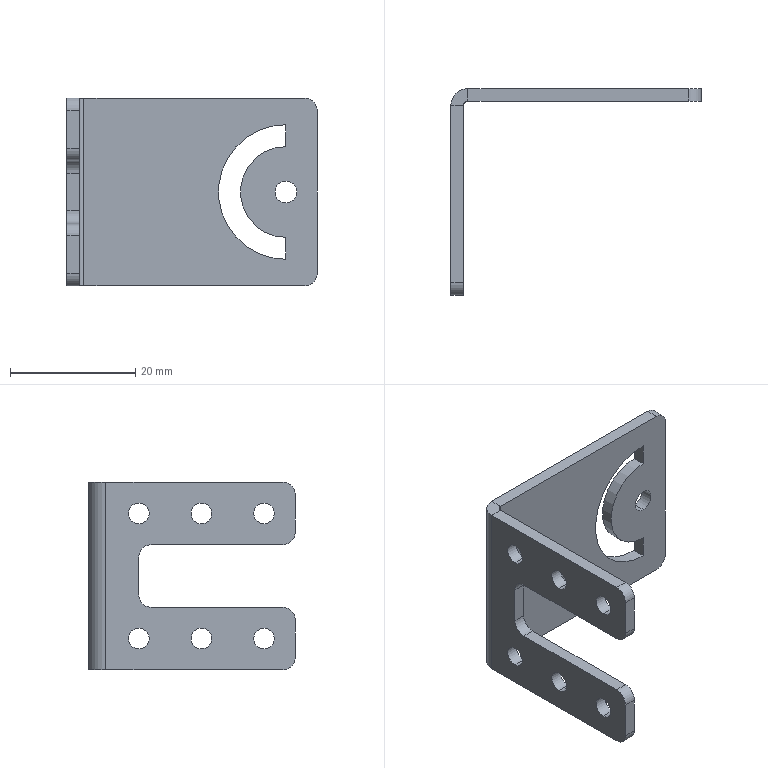Part | SolidWorks | features ICE 3, EdgeFlange 1, Fillet 1, FlatPattern 1, HoleWzd 1, SMBaseFlange 1, SheetMetal 1 | 1 solid | 44 faces | box 40 x 33 x 30 mm | volume 3389 mm3 | cylinder 26 | plane 18 | commonest cylinder face diameters 3.3 x12 4 x8 3.5 x2 1.473 x1 5.473 x1 14.5 x1
STEP:
#1=CARTESIAN_POINT('',(-20.,-18.,-8.35));
#2=VERTEX_POINT('',#1);
#3=CARTESIAN_POINT('',(-20.,-18.,-11.65));
#4=VERTEX_POINT('',#3);
#5=CARTESIAN_POINT('',(-20.,-18.,-10.));
#6=DIRECTION('',(1.,0.,0.));
#7=DIRECTION('',(0.,0.,-1.));
#8=AXIS2_PLACEMENT_3D('',#5,#6,#7);
#9=CIRCLE('',#8,1.65);
#10=EDGE_CURVE('',#2,#4,#9,.T.);
#11=ORIENTED_EDGE('',*,*,#10,.F.);
#12=CARTESIAN_POINT('',(-18.,-18.,-8.35));
#13=VERTEX_POINT('',#12);
#14=CARTESIAN_POINT('',(-18.,-18.,-8.35));
#15=DIRECTION('',(1.,0.,0.));
#16=VECTOR('',#15,1000.);
#17=LINE('',#14,#16);
#18=EDGE_CURVE('',#2,#13,#17,.T.);
#19=ORIENTED_EDGE('',*,*,#18,.T.);
#20=CARTESIAN_POINT('',(-18.,-18.,-11.65));
#21=VERTEX_POINT('',#20);
#22=CARTESIAN_POINT('',(-18.,-18.,-10.));
#23=DIRECTION('',(1.,0.,0.));
#24=DIRECTION('',(0.,0.,-1.));
#25=AXIS2_PLACEMENT_3D('',#22,#23,#24);
#26=CIRCLE('',#25,1.65);
#27=EDGE_CURVE('',#13,#21,#26,.T.);
#28=ORIENTED_EDGE('',*,*,#27,.T.);
#29=CARTESIAN_POINT('',(-18.,-18.,-11.65));
#30=DIRECTION('',(1.,0.,0.));
#31=VECTOR('',#30,1000.);
#32=LINE('',#29,#31);
#33=EDGE_CURVE('',#4,#21,#32,.T.);
#34=ORIENTED_EDGE('',*,*,#33,.F.);
#35=EDGE_LOOP('',(#11,#19,#28,#34));
#36=FACE_OUTER_BOUND('',#35,.T.);
#37=CARTESIAN_POINT('',(-18.,-18.,-10.));
#38=DIRECTION('',(1.,0.,0.));
#39=DIRECTION('',(0.,0.,-1.));
#40=AXIS2_PLACEMENT_3D('',#37,#38,#39);
#41=CYLINDRICAL_SURFACE('',#40,1.65);
#42=ADVANCED_FACE('',(#36),#41,.F.);
#43=CARTESIAN_POINT('',(-20.,-18.,11.65));
#44=VERTEX_POINT('',#43);
#45=CARTESIAN_POINT('',(-20.,-18.,8.35));
#46=VERTEX_POINT('',#45);
#47=CARTESIAN_POINT('',(-20.,-18.,10.));
#48=DIRECTION('',(1.,0.,0.));
#49=DIRECTION('',(0.,0.,-1.));
#50=AXIS2_PLACEMENT_3D('',#47,#48,#49);
#51=CIRCLE('',#50,1.65);
#52=EDGE_CURVE('',#44,#46,#51,.T.);
#53=ORIENTED_EDGE('',*,*,#52,.F.);
#54=CARTESIAN_POINT('',(-18.,-18.,11.65));
#55=VERTEX_POINT('',#54);
#56=CARTESIAN_POINT('',(-18.,-18.,11.65));
#57=DIRECTION('',(1.,0.,0.));
#58=VECTOR('',#57,1000.);
#59=LINE('',#56,#58);
#60=EDGE_CURVE('',#44,#55,#59,.T.);
#61=ORIENTED_EDGE('',*,*,#60,.T.);
#62=CARTESIAN_POINT('',(-18.,-18.,8.35));
#63=VERTEX_POINT('',#62);
#64=CARTESIAN_POINT('',(-18.,-18.,10.));
#65=DIRECTION('',(1.,0.,0.));
#66=DIRECTION('',(0.,0.,-1.));
#67=AXIS2_PLACEMENT_3D('',#64,#65,#66);
#68=CIRCLE('',#67,1.65);
#69=EDGE_CURVE('',#55,#63,#68,.T.);
#70=ORIENTED_EDGE('',*,*,#69,.T.);
#71=CARTESIAN_POINT('',(-18.,-18.,8.35));
#72=DIRECTION('',(1.,0.,0.));
#73=VECTOR('',#72,1000.);
#74=LINE('',#71,#73);
#75=EDGE_CURVE('',#46,#63,#74,.T.);
#76=ORIENTED_EDGE('',*,*,#75,.F.);
#77=EDGE_LOOP('',(#53,#61,#70,#76));
#78=FACE_OUTER_BOUND('',#77,.T.);
#79=CARTESIAN_POINT('',(-18.,-18.,10.));
#80=DIRECTION('',(1.,0.,0.));
#81=DIRECTION('',(0.,0.,-1.));
#82=AXIS2_PLACEMENT_3D('',#79,#80,#81);
#83=CYLINDRICAL_SURFACE('',#82,1.65);
#84=ADVANCED_FACE('',(#78),#83,.F.);
#85=CARTESIAN_POINT('',(-20.,-8.,-8.35));
#86=VERTEX_POINT('',#85);
#87=CARTESIAN_POINT('',(-20.,-8.,-11.65));
#88=VERTEX_POINT('',#87);
#89=CARTESIAN_POINT('',(-20.,-8.,-10.));
#90=DIRECTION('',(1.,0.,0.));
#91=DIRECTION('',(0.,0.,-1.));
#92=AXIS2_PLACEMENT_3D('',#89,#90,#91);
#93=CIRCLE('',#92,1.65);
#94=EDGE_CURVE('',#86,#88,#93,.T.);
#95=ORIENTED_EDGE('',*,*,#94,.F.);
#96=CARTESIAN_POINT('',(-18.,-8.,-8.35));
#97=VERTEX_POINT('',#96);
#98=CARTESIAN_POINT('',(-18.,-8.,-8.35));
#99=DIRECTION('',(1.,0.,0.));
#100=VECTOR('',#99,1000.);
#101=LINE('',#98,#100);
#102=EDGE_CURVE('',#86,#97,#101,.T.);
#103=ORIENTED_EDGE('',*,*,#102,.T.);
#104=CARTESIAN_POINT('',(-18.,-8.,-11.65));
#105=VERTEX_POINT('',#104);
#106=CARTESIAN_POINT('',(-18.,-8.,-10.));
#107=DIRECTION('',(1.,0.,0.));
#108=DIRECTION('',(0.,0.,-1.));
#109=AXIS2_PLACEMENT_3D('',#106,#107,#108);
#110=CIRCLE('',#109,1.65);
#111=EDGE_CURVE('',#97,#105,#110,.T.);
#112=ORIENTED_EDGE('',*,*,#111,.T.);
#113=CARTESIAN_POINT('',(-18.,-8.,-11.65));
#114=DIRECTION('',(1.,0.,0.));
#115=VECTOR('',#114,1000.);
#116=LINE('',#113,#115);
#117=EDGE_CURVE('',#88,#105,#116,.T.);
#118=ORIENTED_EDGE('',*,*,#117,.F.);
#119=EDGE_LOOP('',(#95,#103,#112,#118));
#120=FACE_OUTER_BOUND('',#119,.T.);
#121=CARTESIAN_POINT('',(-18.,-8.,-10.));
#122=DIRECTION('',(1.,0.,0.));
#123=DIRECTION('',(0.,0.,-1.));
#124=AXIS2_PLACEMENT_3D('',#121,#122,#123);
#125=CYLINDRICAL_SURFACE('',#124,1.65);
#126=ADVANCED_FACE('',(#120),#125,.F.);
#127=CARTESIAN_POINT('',(-20.,-28.,-8.35));
#128=VERTEX_POINT('',#127);
#129=CARTESIAN_POINT('',(-20.,-28.,-11.65));
#130=VERTEX_POINT('',#129);
#131=CARTESIAN_POINT('',(-20.,-28.,-10.));
#132=DIRECTION('',(1.,0.,0.));
#133=DIRECTION('',(0.,0.,-1.));
#134=AXIS2_PLACEMENT_3D('',#131,#132,#133);
#135=CIRCLE('',#134,1.65);
#136=EDGE_CURVE('',#128,#130,#135,.T.);
#137=ORIENTED_EDGE('',*,*,#136,.F.);
#138=CARTESIAN_POINT('',(-18.,-28.,-8.35));
#139=VERTEX_POINT('',#138);
#140=CARTESIAN_POINT('',(-18.,-28.,-8.35));
#141=DIRECTION('',(1.,0.,0.));
#142=VECTOR('',#141,1000.);
#143=LINE('',#140,#142);
#144=EDGE_CURVE('',#128,#139,#143,.T.);
#145=ORIENTED_EDGE('',*,*,#144,.T.);
#146=CARTESIAN_POINT('',(-18.,-28.,-11.65));
#147=VERTEX_POINT('',#146);
#148=CARTESIAN_POINT('',(-18.,-28.,-10.));
#149=DIRECTION('',(1.,0.,0.));
#150=DIRECTION('',(0.,0.,-1.));
#151=AXIS2_PLACEMENT_3D('',#148,#149,#150);
#152=CIRCLE('',#151,1.65);
#153=EDGE_CURVE('',#139,#147,#152,.T.);
#154=ORIENTED_EDGE('',*,*,#153,.T.);
#155=CARTESIAN_POINT('',(-18.,-28.,-11.65));
#156=DIRECTION('',(1.,0.,0.));
#157=VECTOR('',#156,1000.);
#158=LINE('',#155,#157);
#159=EDGE_CURVE('',#130,#147,#158,.T.);
#160=ORIENTED_EDGE('',*,*,#159,.F.);
#161=EDGE_LOOP('',(#137,#145,#154,#160));
#162=FACE_OUTER_BOUND('',#161,.T.);
#163=CARTESIAN_POINT('',(-18.,-28.,-10.));
#164=DIRECTION('',(1.,0.,0.));
#165=DIRECTION('',(0.,0.,-1.));
#166=AXIS2_PLACEMENT_3D('',#163,#164,#165);
#167=CYLINDRICAL_SURFACE('',#166,1.65);
#168=ADVANCED_FACE('',(#162),#167,.F.);
#169=CARTESIAN_POINT('',(-20.,-8.,11.65));
#170=VERTEX_POINT('',#169);
#171=CARTESIAN_POINT('',(-20.,-8.,8.35));
#172=VERTEX_POINT('',#171);
#173=CARTESIAN_POINT('',(-20.,-8.,10.));
#174=DIRECTION('',(1.,0.,0.));
#175=DIRECTION('',(0.,0.,-1.));
#176=AXIS2_PLACEMENT_3D('',#173,#174,#175);
#177=CIRCLE('',#176,1.65);
#178=EDGE_CURVE('',#170,#172,#177,.T.);
#179=ORIENTED_EDGE('',*,*,#178,.F.);
#180=CARTESIAN_POINT('',(-18.,-8.,11.65));
#181=VERTEX_POINT('',#180);
#182=CARTESIAN_POINT('',(-18.,-8.,11.65));
#183=DIRECTION('',(1.,0.,0.));
#184=VECTOR('',#183,1000.);
#185=LINE('',#182,#184);
#186=EDGE_CURVE('',#170,#181,#185,.T.);
#187=ORIENTED_EDGE('',*,*,#186,.T.);
#188=CARTESIAN_POINT('',(-18.,-8.,8.35));
#189=VERTEX_POINT('',#188);
#190=CARTESIAN_POINT('',(-18.,-8.,10.));
#191=DIRECTION('',(1.,0.,0.));
#192=DIRECTION('',(0.,0.,-1.));
#193=AXIS2_PLACEMENT_3D('',#190,#191,#192);
#194=CIRCLE('',#193,1.65);
#195=EDGE_CURVE('',#181,#189,#194,.T.);
#196=ORIENTED_EDGE('',*,*,#195,.T.);
#197=CARTESIAN_POINT('',(-18.,-8.,8.35));
#198=DIRECTION('',(1.,0.,0.));
#199=VECTOR('',#198,1000.);
#200=LINE('',#197,#199);
#201=EDGE_CURVE('',#172,#189,#200,.T.);
#202=ORIENTED_EDGE('',*,*,#201,.F.);
#203=EDGE_LOOP('',(#179,#187,#196,#202));
#204=FACE_OUTER_BOUND('',#203,.T.);
#205=CARTESIAN_POINT('',(-18.,-8.,10.));
#206=DIRECTION('',(1.,0.,0.));
#207=DIRECTION('',(0.,0.,-1.));
#208=AXIS2_PLACEMENT_3D('',#205,#206,#207);
#209=CYLINDRICAL_SURFACE('',#208,1.65);
#210=ADVANCED_FACE('',(#204),#209,.F.);
#211=CARTESIAN_POINT('',(-20.,-28.,11.65));
#212=VERTEX_POINT('',#211);
#213=CARTESIAN_POINT('',(-20.,-28.,8.35));
#214=VERTEX_POINT('',#213);
#215=CARTESIAN_POINT('',(-20.,-28.,10.));
#216=DIRECTION('',(1.,0.,0.));
#217=DIRECTION('',(0.,0.,-1.));
#218=AXIS2_PLACEMENT_3D('',#215,#216,#217);
#219=CIRCLE('',#218,1.65);
#220=EDGE_CURVE('',#212,#214,#219,.T.);
#221=ORIENTED_EDGE('',*,*,#220,.F.);
#222=CARTESIAN_POINT('',(-18.,-28.,11.65));
#223=VERTEX_POINT('',#222);
#224=CARTESIAN_POINT('',(-18.,-28.,11.65));
#225=DIRECTION('',(1.,0.,0.));
#226=VECTOR('',#225,1000.);
#227=LINE('',#224,#226);
#228=EDGE_CURVE('',#212,#223,#227,.T.);
#229=ORIENTED_EDGE('',*,*,#228,.T.);
#230=CARTESIAN_POINT('',(-18.,-28.,8.35));
#231=VERTEX_POINT('',#230);
#232=CARTESIAN_POINT('',(-18.,-28.,10.));
#233=DIRECTION('',(1.,0.,0.));
#234=DIRECTION('',(0.,0.,-1.));
#235=AXIS2_PLACEMENT_3D('',#232,#233,#234);
#236=CIRCLE('',#235,1.65);
#237=EDGE_CURVE('',#223,#231,#236,.T.);
#238=ORIENTED_EDGE('',*,*,#237,.T.);
#239=CARTESIAN_POINT('',(-18.,-28.,8.35));
#240=DIRECTION('',(1.,0.,0.));
#241=VECTOR('',#240,1000.);
#242=LINE('',#239,#241);
#243=EDGE_CURVE('',#214,#231,#242,.T.);
#244=ORIENTED_EDGE('',*,*,#243,.F.);
#245=EDGE_LOOP('',(#221,#229,#238,#244));
#246=FACE_OUTER_BOUND('',#245,.T.);
#247=CARTESIAN_POINT('',(-18.,-28.,10.));
#248=DIRECTION('',(1.,0.,0.));
#249=DIRECTION('',(0.,0.,-1.));
#250=AXIS2_PLACEMENT_3D('',#247,#248,#249);
#251=CYLINDRICAL_SURFACE('',#250,1.65);
#252=ADVANCED_FACE('',(#246),#251,.F.);
#253=CARTESIAN_POINT('',(15.,0.,1.75));
#254=VERTEX_POINT('',#253);
#255=CARTESIAN_POINT('',(15.,0.,-1.75));
#256=VERTEX_POINT('',#255);
#257=CARTESIAN_POINT('',(15.,0.,0.));
#258=DIRECTION('',(0.,-1.,0.));
#259=DIRECTION('',(0.,0.,-1.));
#260=AXIS2_PLACEMENT_3D('',#257,#258,#259);
#261=CIRCLE('',#260,1.75);
#262=EDGE_CURVE('',#254,#256,#261,.T.);
#263=ORIENTED_EDGE('',*,*,#262,.F.);
#264=CARTESIAN_POINT('',(15.,-2.,1.75));
#265=VERTEX_POINT('',#264);
#266=CARTESIAN_POINT('',(15.,0.,1.75));
#267=DIRECTION('',(0.,-1.,0.));
#268=VECTOR('',#267,1000.);
#269=LINE('',#266,#268);
#270=EDGE_CURVE('',#254,#265,#269,.T.);
#271=ORIENTED_EDGE('',*,*,#270,.T.);
#272=CARTESIAN_POINT('',(15.,-2.,-1.75));
#273=VERTEX_POINT('',#272);
#274=CARTESIAN_POINT('',(15.,-2.,0.));
#275=DIRECTION('',(0.,-1.,0.));
#276=DIRECTION('',(0.,0.,-1.));
#277=AXIS2_PLACEMENT_3D('',#274,#275,#276);
#278=CIRCLE('',#277,1.75);
#279=EDGE_CURVE('',#265,#273,#278,.T.);
#280=ORIENTED_EDGE('',*,*,#279,.T.);
#281=CARTESIAN_POINT('',(15.,0.,-1.75));
#282=DIRECTION('',(0.,-1.,0.));
#283=VECTOR('',#282,1000.);
#284=LINE('',#281,#283);
#285=EDGE_CURVE('',#256,#273,#284,.T.);
#286=ORIENTED_EDGE('',*,*,#285,.F.);
#287=EDGE_LOOP('',(#263,#271,#280,#286));
#288=FACE_OUTER_BOUND('',#287,.T.);
#289=CARTESIAN_POINT('',(15.,0.,0.));
#290=DIRECTION('',(0.,-1.,0.));
#291=DIRECTION('',(0.,0.,-1.));
#292=AXIS2_PLACEMENT_3D('',#289,#290,#291);
#293=CYLINDRICAL_SURFACE('',#292,1.75);
#294=ADVANCED_FACE('',(#288),#293,.F.);
#295=CARTESIAN_POINT('',(-18.,-33.,-7.));
#296=VERTEX_POINT('',#295);
#297=CARTESIAN_POINT('',(-18.,-33.,-13.));
#298=VERTEX_POINT('',#297);
#299=CARTESIAN_POINT('',(-18.,-33.,0.));
#300=DIRECTION('',(0.,0.,-1.));
#301=VECTOR('',#300,1000.);
#302=LINE('',#299,#301);
#303=EDGE_CURVE('',#296,#298,#302,.T.);
#304=ORIENTED_EDGE('',*,*,#303,.F.);
#305=CARTESIAN_POINT('',(-20.,-33.,-7.));
#306=VERTEX_POINT('',#305);
#307=CARTESIAN_POINT('',(-20.,-33.,-7.));
#308=DIRECTION('',(-1.,0.,0.));
#309=VECTOR('',#308,1000.);
#310=LINE('',#307,#309);
#311=EDGE_CURVE('',#296,#306,#310,.T.);
#312=ORIENTED_EDGE('',*,*,#311,.T.);
#313=CARTESIAN_POINT('',(-20.,-33.,-13.));
#314=VERTEX_POINT('',#313);
#315=CARTESIAN_POINT('',(-20.,-33.,-15.));
#316=DIRECTION('',(0.,0.,-1.));
#317=VECTOR('',#316,1000.);
#318=LINE('',#315,#317);
#319=EDGE_CURVE('',#306,#314,#318,.T.);
#320=ORIENTED_EDGE('',*,*,#319,.T.);
#321=CARTESIAN_POINT('',(-20.,-33.,-13.));
#322=DIRECTION('',(1.,0.,0.));
#323=VECTOR('',#322,1000.);
#324=LINE('',#321,#323);
#325=EDGE_CURVE('',#314,#298,#324,.T.);
#326=ORIENTED_EDGE('',*,*,#325,.T.);
#327=EDGE_LOOP('',(#304,#312,#320,#326));
#328=FACE_OUTER_BOUND('',#327,.T.);
#329=CARTESIAN_POINT('',(-20.,-33.,-15.));
#330=DIRECTION('',(0.,-1.,0.));
#331=DIRECTION('',(1.,0.,0.));
#332=AXIS2_PLACEMENT_3D('',#329,#330,#331);
#333=PLANE('',#332);
#334=ADVANCED_FACE('',(#328),#333,.T.);
#335=CARTESIAN_POINT('',(18.,0.,-15.));
#336=VERTEX_POINT('',#335);
#337=CARTESIAN_POINT('',(-17.263,0.,-15.));
#338=VERTEX_POINT('',#337);
#339=CARTESIAN_POINT('',(-20.,0.,-15.));
#340=DIRECTION('',(-1.,0.,0.));
#341=VECTOR('',#340,1000.);
#342=LINE('',#339,#341);
#343=EDGE_CURVE('',#336,#338,#342,.T.);
#344=ORIENTED_EDGE('',*,*,#343,.F.);
#345=CARTESIAN_POINT('',(18.,-2.,-15.));
#346=VERTEX_POINT('',#345);
#347=CARTESIAN_POINT('',(18.,-2.,-15.));
#348=DIRECTION('',(0.,-1.,0.));
#349=VECTOR('',#348,1000.);
#350=LINE('',#347,#349);
#351=EDGE_CURVE('',#336,#346,#350,.T.);
#352=ORIENTED_EDGE('',*,*,#351,.T.);
#353=CARTESIAN_POINT('',(-17.263,-2.,-15.));
#354=VERTEX_POINT('',#353);
#355=CARTESIAN_POINT('',(-20.,-2.,-15.));
#356=DIRECTION('',(-1.,0.,0.));
#357=VECTOR('',#356,1000.);
#358=LINE('',#355,#357);
#359=EDGE_CURVE('',#346,#354,#358,.T.);
#360=ORIENTED_EDGE('',*,*,#359,.T.);
#361=CARTESIAN_POINT('',(-17.263,-2.,-15.));
#362=DIRECTION('',(0.,1.,0.));
#363=VECTOR('',#362,1000.);
#364=LINE('',#361,#363);
#365=EDGE_CURVE('',#354,#338,#364,.T.);
#366=ORIENTED_EDGE('',*,*,#365,.T.);
#367=EDGE_LOOP('',(#344,#352,#360,#366));
#368=FACE_OUTER_BOUND('',#367,.T.);
#369=CARTESIAN_POINT('',(-20.,-2.,-15.));
#370=DIRECTION('',(0.,0.,-1.));
#371=DIRECTION('',(-1.,0.,0.));
#372=AXIS2_PLACEMENT_3D('',#369,#370,#371);
#373=PLANE('',#372);
#374=ADVANCED_FACE('',(#368),#373,.T.);
#375=CARTESIAN_POINT('',(15.,-2.,-7.25));
#376=VERTEX_POINT('',#375);
#377=CARTESIAN_POINT('',(15.,-2.,7.25));
#378=VERTEX_POINT('',#377);
#379=CARTESIAN_POINT('',(15.,-2.,0.));
#380=DIRECTION('',(0.,1.,0.));
#381=DIRECTION('',(0.,0.,-1.));
#382=AXIS2_PLACEMENT_3D('',#379,#380,#381);
#383=CIRCLE('',#382,7.25);
#384=EDGE_CURVE('',#376,#378,#383,.T.);
#385=ORIENTED_EDGE('',*,*,#384,.F.);
#386=CARTESIAN_POINT('',(15.,-2.,-10.75));
#387=VERTEX_POINT('',#386);
#388=CARTESIAN_POINT('',(15.,-2.,-10.75));
#389=DIRECTION('',(0.,0.,1.));
#390=VECTOR('',#389,1000.);
#391=LINE('',#388,#390);
#392=EDGE_CURVE('',#387,#376,#391,.T.);
#393=ORIENTED_EDGE('',*,*,#392,.F.);
#394=CARTESIAN_POINT('',(15.,-2.,10.75));
#395=VERTEX_POINT('',#394);
#396=CARTESIAN_POINT('',(15.,-2.,0.));
#397=DIRECTION('',(0.,-1.,0.));
#398=DIRECTION('',(0.,0.,-1.));
#399=AXIS2_PLACEMENT_3D('',#396,#397,#398);
#400=CIRCLE('',#399,10.75);
#401=EDGE_CURVE('',#395,#387,#400,.T.);
#402=ORIENTED_EDGE('',*,*,#401,.F.);
#403=CARTESIAN_POINT('',(15.,-2.,10.75));
#404=DIRECTION('',(0.,0.,1.));
#405=VECTOR('',#404,1000.);
#406=LINE('',#403,#405);
#407=EDGE_CURVE('',#378,#395,#406,.T.);
#408=ORIENTED_EDGE('',*,*,#407,.F.);
#409=EDGE_LOOP('',(#385,#393,#402,#408));
#410=FACE_BOUND('',#409,.T.);
#411=CARTESIAN_POINT('',(15.,-2.,0.));
#412=DIRECTION('',(0.,-1.,0.));
#413=DIRECTION('',(0.,0.,-1.));
#414=AXIS2_PLACEMENT_3D('',#411,#412,#413);
#415=CIRCLE('',#414,1.75);
#416=EDGE_CURVE('',#273,#265,#415,.T.);
#417=ORIENTED_EDGE('',*,*,#416,.F.);
#418=ORIENTED_EDGE('',*,*,#279,.F.);
#419=EDGE_LOOP('',(#417,#418));
#420=FACE_BOUND('',#419,.T.);
#421=ORIENTED_EDGE('',*,*,#359,.F.);
#422=CARTESIAN_POINT('',(20.,-2.,-13.));
#423=VERTEX_POINT('',#422);
#424=CARTESIAN_POINT('',(18.,-2.,-13.));
#425=DIRECTION('',(0.,-1.,0.));
#426=DIRECTION('',(0.,0.,1.));
#427=AXIS2_PLACEMENT_3D('',#424,#425,#426);
#428=CIRCLE('',#427,2.);
#429=EDGE_CURVE('',#346,#423,#428,.T.);
#430=ORIENTED_EDGE('',*,*,#429,.T.);
#431=CARTESIAN_POINT('',(20.,-2.,13.));
#432=VERTEX_POINT('',#431);
#433=CARTESIAN_POINT('',(20.,-2.,-15.));
#434=DIRECTION('',(0.,0.,-1.));
#435=VECTOR('',#434,1000.);
#436=LINE('',#433,#435);
#437=EDGE_CURVE('',#432,#423,#436,.T.);
#438=ORIENTED_EDGE('',*,*,#437,.F.);
#439=CARTESIAN_POINT('',(18.,-2.,15.));
#440=VERTEX_POINT('',#439);
#441=CARTESIAN_POINT('',(18.,-2.,13.));
#442=DIRECTION('',(0.,-1.,0.));
#443=DIRECTION('',(0.,0.,1.));
#444=AXIS2_PLACEMENT_3D('',#441,#442,#443);
#445=CIRCLE('',#444,2.);
#446=EDGE_CURVE('',#432,#440,#445,.T.);
#447=ORIENTED_EDGE('',*,*,#446,.T.);
#448=CARTESIAN_POINT('',(-17.263,-2.,15.));
#449=VERTEX_POINT('',#448);
#450=CARTESIAN_POINT('',(-20.,-2.,15.));
#451=DIRECTION('',(1.,0.,0.));
#452=VECTOR('',#451,1000.);
#453=LINE('',#450,#452);
#454=EDGE_CURVE('',#449,#440,#453,.T.);
#455=ORIENTED_EDGE('',*,*,#454,.F.);
#456=CARTESIAN_POINT('',(-17.263,-2.,-15.));
#457=DIRECTION('',(0.,0.,1.));
#458=VECTOR('',#457,1000.);
#459=LINE('',#456,#458);
#460=EDGE_CURVE('',#354,#449,#459,.T.);
#461=ORIENTED_EDGE('',*,*,#460,.F.);
#462=EDGE_LOOP('',(#421,#430,#438,#447,#455,#461));
#463=FACE_OUTER_BOUND('',#462,.T.);
#464=CARTESIAN_POINT('',(0.,-2.,0.));
#465=DIRECTION('',(0.,1.,0.));
#466=DIRECTION('',(0.,0.,1.));
#467=AXIS2_PLACEMENT_3D('',#464,#465,#466);
#468=PLANE('',#467);
#469=ADVANCED_FACE('',(#410,#420,#463),#468,.F.);
#470=CARTESIAN_POINT('',(15.,0.,-7.25));
#471=VERTEX_POINT('',#470);
#472=CARTESIAN_POINT('',(15.,0.,7.25));
#473=VERTEX_POINT('',#472);
#474=CARTESIAN_POINT('',(15.,0.,0.));
#475=DIRECTION('',(0.,1.,0.));
#476=DIRECTION('',(0.,0.,-1.));
#477=AXIS2_PLACEMENT_3D('',#474,#475,#476);
#478=CIRCLE('',#477,7.25);
#479=EDGE_CURVE('',#471,#473,#478,.T.);
#480=ORIENTED_EDGE('',*,*,#479,.T.);
#481=CARTESIAN_POINT('',(15.,0.,10.75));
#482=VERTEX_POINT('',#481);
#483=CARTESIAN_POINT('',(15.,0.,10.75));
#484=DIRECTION('',(0.,0.,1.));
#485=VECTOR('',#484,1000.);
#486=LINE('',#483,#485);
#487=EDGE_CURVE('',#473,#482,#486,.T.);
#488=ORIENTED_EDGE('',*,*,#487,.T.);
#489=CARTESIAN_POINT('',(15.,0.,-10.75));
#490=VERTEX_POINT('',#489);
#491=CARTESIAN_POINT('',(15.,0.,0.));
#492=DIRECTION('',(0.,-1.,0.));
#493=DIRECTION('',(0.,0.,-1.));
#494=AXIS2_PLACEMENT_3D('',#491,#492,#493);
#495=CIRCLE('',#494,10.75);
#496=EDGE_CURVE('',#482,#490,#495,.T.);
#497=ORIENTED_EDGE('',*,*,#496,.T.);
#498=CARTESIAN_POINT('',(15.,0.,-10.75));
#499=DIRECTION('',(0.,0.,1.));
#500=VECTOR('',#499,1000.);
#501=LINE('',#498,#500);
#502=EDGE_CURVE('',#490,#471,#501,.T.);
#503=ORIENTED_EDGE('',*,*,#502,.T.);
#504=EDGE_LOOP('',(#480,#488,#497,#503));
#505=FACE_BOUND('',#504,.T.);
#506=CARTESIAN_POINT('',(15.,0.,0.));
#507=DIRECTION('',(0.,-1.,0.));
#508=DIRECTION('',(0.,0.,-1.));
#509=AXIS2_PLACEMENT_3D('',#506,#507,#508);
#510=CIRCLE('',#509,1.75);
#511=EDGE_CURVE('',#256,#254,#510,.T.);
#512=ORIENTED_EDGE('',*,*,#511,.T.);
#513=ORIENTED_EDGE('',*,*,#262,.T.);
#514=EDGE_LOOP('',(#512,#513));
#515=FACE_BOUND('',#514,.T.);
#516=CARTESIAN_POINT('',(20.,0.,13.));
#517=VERTEX_POINT('',#516);
#518=CARTESIAN_POINT('',(20.,0.,-13.));
#519=VERTEX_POINT('',#518);
#520=CARTESIAN_POINT('',(20.,0.,-15.));
#521=DIRECTION('',(0.,0.,-1.));
#522=VECTOR('',#521,1000.);
#523=LINE('',#520,#522);
#524=EDGE_CURVE('',#517,#519,#523,.T.);
#525=ORIENTED_EDGE('',*,*,#524,.T.);
#526=CARTESIAN_POINT('',(18.,0.,-13.));
#527=DIRECTION('',(0.,1.,0.));
#528=DIRECTION('',(0.,0.,1.));
#529=AXIS2_PLACEMENT_3D('',#526,#527,#528);
#530=CIRCLE('',#529,2.);
#531=EDGE_CURVE('',#519,#336,#530,.T.);
#532=ORIENTED_EDGE('',*,*,#531,.T.);
#533=ORIENTED_EDGE('',*,*,#343,.T.);
#534=CARTESIAN_POINT('',(-17.263,0.,15.));
#535=VERTEX_POINT('',#534);
#536=CARTESIAN_POINT('',(-17.263,0.,-15.));
#537=DIRECTION('',(0.,0.,1.));
#538=VECTOR('',#537,1000.);
#539=LINE('',#536,#538);
#540=EDGE_CURVE('',#338,#535,#539,.T.);
#541=ORIENTED_EDGE('',*,*,#540,.T.);
#542=CARTESIAN_POINT('',(18.,0.,15.));
#543=VERTEX_POINT('',#542);
#544=CARTESIAN_POINT('',(-20.,0.,15.));
#545=DIRECTION('',(1.,0.,0.));
#546=VECTOR('',#545,1000.);
#547=LINE('',#544,#546);
#548=EDGE_CURVE('',#535,#543,#547,.T.);
#549=ORIENTED_EDGE('',*,*,#548,.T.);
#550=CARTESIAN_POINT('',(18.,0.,13.));
#551=DIRECTION('',(0.,1.,0.));
#552=DIRECTION('',(0.,0.,1.));
#553=AXIS2_PLACEMENT_3D('',#550,#551,#552);
#554=CIRCLE('',#553,2.);
#555=EDGE_CURVE('',#543,#517,#554,.T.);
#556=ORIENTED_EDGE('',*,*,#555,.T.);
#557=EDGE_LOOP('',(#525,#532,#533,#541,#549,#556));
#558=FACE_OUTER_BOUND('',#557,.T.);
#559=CARTESIAN_POINT('',(0.,0.,0.));
#560=DIRECTION('',(0.,1.,0.));
#561=DIRECTION('',(0.,0.,1.));
#562=AXIS2_PLACEMENT_3D('',#559,#560,#561);
#563=PLANE('',#562);
#564=ADVANCED_FACE('',(#505,#515,#558),#563,.T.);
#565=ORIENTED_EDGE('',*,*,#437,.T.);
#566=CARTESIAN_POINT('',(20.,-2.,-13.));
#567=DIRECTION('',(0.,1.,0.));
#568=VECTOR('',#567,1000.);
#569=LINE('',#566,#568);
#570=EDGE_CURVE('',#423,#519,#569,.T.);
#571=ORIENTED_EDGE('',*,*,#570,.T.);
#572=ORIENTED_EDGE('',*,*,#524,.F.);
#573=CARTESIAN_POINT('',(20.,-2.,13.));
#574=DIRECTION('',(0.,-1.,0.));
#575=VECTOR('',#574,1000.);
#576=LINE('',#573,#575);
#577=EDGE_CURVE('',#517,#432,#576,.T.);
#578=ORIENTED_EDGE('',*,*,#577,.T.);
#579=EDGE_LOOP('',(#565,#571,#572,#578));
#580=FACE_OUTER_BOUND('',#579,.T.);
#581=CARTESIAN_POINT('',(20.,-2.,-15.));
#582=DIRECTION('',(1.,0.,0.));
#583=DIRECTION('',(0.,0.,-1.));
#584=AXIS2_PLACEMENT_3D('',#581,#582,#583);
#585=PLANE('',#584);
#586=ADVANCED_FACE('',(#580),#585,.T.);
#587=ORIENTED_EDGE('',*,*,#454,.T.);
#588=CARTESIAN_POINT('',(18.,-2.,15.));
#589=DIRECTION('',(0.,1.,0.));
#590=VECTOR('',#589,1000.);
#591=LINE('',#588,#590);
#592=EDGE_CURVE('',#440,#543,#591,.T.);
#593=ORIENTED_EDGE('',*,*,#592,.T.);
#594=ORIENTED_EDGE('',*,*,#548,.F.);
#595=CARTESIAN_POINT('',(-17.263,-2.,15.));
#596=DIRECTION('',(0.,1.,0.));
#597=VECTOR('',#596,1000.);
#598=LINE('',#595,#597);
#599=EDGE_CURVE('',#449,#535,#598,.T.);
#600=ORIENTED_EDGE('',*,*,#599,.F.);
#601=EDGE_LOOP('',(#587,#593,#594,#600));
#602=FACE_OUTER_BOUND('',#601,.T.);
#603=CARTESIAN_POINT('',(-20.,-2.,15.));
#604=DIRECTION('',(0.,0.,1.));
#605=DIRECTION('',(1.,0.,0.));
#606=AXIS2_PLACEMENT_3D('',#603,#604,#605);
#607=PLANE('',#606);
#608=ADVANCED_FACE('',(#602),#607,.T.);
#609=ORIENTED_EDGE('',*,*,#270,.F.);
#610=ORIENTED_EDGE('',*,*,#511,.F.);
#611=ORIENTED_EDGE('',*,*,#285,.T.);
#612=ORIENTED_EDGE('',*,*,#416,.T.);
#613=EDGE_LOOP('',(#609,#610,#611,#612));
#614=FACE_OUTER_BOUND('',#613,.T.);
#615=CARTESIAN_POINT('',(15.,0.,0.));
#616=DIRECTION('',(0.,-1.,0.));
#617=DIRECTION('',(0.,0.,-1.));
#618=AXIS2_PLACEMENT_3D('',#615,#616,#617);
#619=CYLINDRICAL_SURFACE('',#618,1.75);
#620=ADVANCED_FACE('',(#614),#619,.F.);
#621=ORIENTED_EDGE('',*,*,#479,.F.);
#622=CARTESIAN_POINT('',(15.,0.,-7.25));
#623=DIRECTION('',(0.,-1.,0.));
#624=VECTOR('',#623,1000.);
#625=LINE('',#622,#624);
#626=EDGE_CURVE('',#471,#376,#625,.T.);
#627=ORIENTED_EDGE('',*,*,#626,.T.);
#628=ORIENTED_EDGE('',*,*,#384,.T.);
#629=CARTESIAN_POINT('',(15.,0.,7.25));
#630=DIRECTION('',(0.,-1.,0.));
#631=VECTOR('',#630,1000.);
#632=LINE('',#629,#631);
#633=EDGE_CURVE('',#473,#378,#632,.T.);
#634=ORIENTED_EDGE('',*,*,#633,.F.);
#635=EDGE_LOOP('',(#621,#627,#628,#634));
#636=FACE_OUTER_BOUND('',#635,.T.);
#637=CARTESIAN_POINT('',(15.,0.,0.));
#638=DIRECTION('',(0.,-1.,0.));
#639=DIRECTION('',(0.,0.,-1.));
#640=AXIS2_PLACEMENT_3D('',#637,#638,#639);
#641=CYLINDRICAL_SURFACE('',#640,7.25);
#642=ADVANCED_FACE('',(#636),#641,.T.);
#643=ORIENTED_EDGE('',*,*,#496,.F.);
#644=CARTESIAN_POINT('',(15.,0.,10.75));
#645=DIRECTION('',(0.,-1.,0.));
#646=VECTOR('',#645,1000.);
#647=LINE('',#644,#646);
#648=EDGE_CURVE('',#482,#395,#647,.T.);
#649=ORIENTED_EDGE('',*,*,#648,.T.);
#650=ORIENTED_EDGE('',*,*,#401,.T.);
#651=CARTESIAN_POINT('',(15.,0.,-10.75));
#652=DIRECTION('',(0.,-1.,0.));
#653=VECTOR('',#652,1000.);
#654=LINE('',#651,#653);
#655=EDGE_CURVE('',#490,#387,#654,.T.);
#656=ORIENTED_EDGE('',*,*,#655,.F.);
#657=EDGE_LOOP('',(#643,#649,#650,#656));
#658=FACE_OUTER_BOUND('',#657,.T.);
#659=CARTESIAN_POINT('',(15.,0.,0.));
#660=DIRECTION('',(0.,-1.,0.));
#661=DIRECTION('',(0.,0.,-1.));
#662=AXIS2_PLACEMENT_3D('',#659,#660,#661);
#663=CYLINDRICAL_SURFACE('',#662,10.75);
#664=ADVANCED_FACE('',(#658),#663,.F.);
#665=ORIENTED_EDGE('',*,*,#392,.T.);
#666=ORIENTED_EDGE('',*,*,#626,.F.);
#667=ORIENTED_EDGE('',*,*,#502,.F.);
#668=ORIENTED_EDGE('',*,*,#655,.T.);
#669=EDGE_LOOP('',(#665,#666,#667,#668));
#670=FACE_OUTER_BOUND('',#669,.T.);
#671=CARTESIAN_POINT('',(15.,0.,-10.75));
#672=DIRECTION('',(1.,0.,0.));
#673=DIRECTION('',(0.,0.,-1.));
#674=AXIS2_PLACEMENT_3D('',#671,#672,#673);
#675=PLANE('',#674);
#676=ADVANCED_FACE('',(#670),#675,.F.);
#677=ORIENTED_EDGE('',*,*,#407,.T.);
#678=ORIENTED_EDGE('',*,*,#648,.F.);
#679=ORIENTED_EDGE('',*,*,#487,.F.);
#680=ORIENTED_EDGE('',*,*,#633,.T.);
#681=EDGE_LOOP('',(#677,#678,#679,#680));
#682=FACE_OUTER_BOUND('',#681,.T.);
#683=CARTESIAN_POINT('',(15.,0.,10.75));
#684=DIRECTION('',(1.,0.,0.));
#685=DIRECTION('',(0.,0.,-1.));
#686=AXIS2_PLACEMENT_3D('',#683,#684,#685);
#687=PLANE('',#686);
#688=ADVANCED_FACE('',(#682),#687,.F.);
#689=CARTESIAN_POINT('',(-18.,-2.737,15.));
#690=VERTEX_POINT('',#689);
#691=CARTESIAN_POINT('',(-20.,-2.737,15.));
#692=VERTEX_POINT('',#691);
#693=CARTESIAN_POINT('',(-20.,-2.737,15.));
#694=DIRECTION('',(-1.,0.,0.));
#695=VECTOR('',#694,1000.);
#696=LINE('',#693,#695);
#697=EDGE_CURVE('',#690,#692,#696,.T.);
#698=ORIENTED_EDGE('',*,*,#697,.F.);
#699=CARTESIAN_POINT('',(-17.263,-2.737,15.));
#700=DIRECTION('',(0.,0.,1.));
#701=DIRECTION('',(-1.,0.,0.));
#702=AXIS2_PLACEMENT_3D('',#699,#700,#701);
#703=CIRCLE('',#702,0.7366);
#704=EDGE_CURVE('',#449,#690,#703,.T.);
#705=ORIENTED_EDGE('',*,*,#704,.F.);
#706=ORIENTED_EDGE('',*,*,#599,.T.);
#707=CARTESIAN_POINT('',(-17.263,-2.737,15.));
#708=DIRECTION('',(0.,0.,1.));
#709=DIRECTION('',(-1.,0.,0.));
#710=AXIS2_PLACEMENT_3D('',#707,#708,#709);
#711=CIRCLE('',#710,2.737);
#712=EDGE_CURVE('',#535,#692,#711,.T.);
#713=ORIENTED_EDGE('',*,*,#712,.T.);
#714=EDGE_LOOP('',(#698,#705,#706,#713));
#715=FACE_OUTER_BOUND('',#714,.T.);
#716=CARTESIAN_POINT('',(-17.263,-2.737,15.));
#717=DIRECTION('',(0.,0.,1.));
#718=DIRECTION('',(1.,0.,0.));
#719=AXIS2_PLACEMENT_3D('',#716,#717,#718);
#720=PLANE('',#719);
#721=ADVANCED_FACE('',(#715),#720,.T.);
#722=CARTESIAN_POINT('',(-18.,-2.737,-15.));
#723=VERTEX_POINT('',#722);
#724=CARTESIAN_POINT('',(-17.263,-2.737,-15.));
#725=DIRECTION('',(0.,0.,-1.));
#726=DIRECTION('',(-1.,0.,0.));
#727=AXIS2_PLACEMENT_3D('',#724,#725,#726);
#728=CIRCLE('',#727,0.7366);
#729=EDGE_CURVE('',#723,#354,#728,.T.);
#730=ORIENTED_EDGE('',*,*,#729,.F.);
#731=CARTESIAN_POINT('',(-20.,-2.737,-15.));
#732=VERTEX_POINT('',#731);
#733=CARTESIAN_POINT('',(-18.,-2.737,-15.));
#734=DIRECTION('',(-1.,0.,0.));
#735=VECTOR('',#734,1000.);
#736=LINE('',#733,#735);
#737=EDGE_CURVE('',#723,#732,#736,.T.);
#738=ORIENTED_EDGE('',*,*,#737,.T.);
#739=CARTESIAN_POINT('',(-17.263,-2.737,-15.));
#740=DIRECTION('',(0.,0.,-1.));
#741=DIRECTION('',(-1.,0.,0.));
#742=AXIS2_PLACEMENT_3D('',#739,#740,#741);
#743=CIRCLE('',#742,2.737);
#744=EDGE_CURVE('',#732,#338,#743,.T.);
#745=ORIENTED_EDGE('',*,*,#744,.T.);
#746=ORIENTED_EDGE('',*,*,#365,.F.);
#747=EDGE_LOOP('',(#730,#738,#745,#746));
#748=FACE_OUTER_BOUND('',#747,.T.);
#749=CARTESIAN_POINT('',(-17.263,-2.737,-15.));
#750=DIRECTION('',(0.,0.,1.));
#751=DIRECTION('',(1.,0.,0.));
#752=AXIS2_PLACEMENT_3D('',#749,#750,#751);
#753=PLANE('',#752);
#754=ADVANCED_FACE('',(#748),#753,.F.);
#755=ORIENTED_EDGE('',*,*,#540,.F.);
#756=ORIENTED_EDGE('',*,*,#744,.F.);
#757=CARTESIAN_POINT('',(-20.,-2.737,0.));
#758=DIRECTION('',(0.,0.,-1.));
#759=VECTOR('',#758,1000.);
#760=LINE('',#757,#759);
#761=EDGE_CURVE('',#692,#732,#760,.T.);
#762=ORIENTED_EDGE('',*,*,#761,.F.);
#763=ORIENTED_EDGE('',*,*,#712,.F.);
#764=EDGE_LOOP('',(#755,#756,#762,#763));
#765=FACE_OUTER_BOUND('',#764,.T.);
#766=CARTESIAN_POINT('',(-17.263,-2.737,-15.));
#767=DIRECTION('',(0.,0.,-1.));
#768=DIRECTION('',(-1.,0.,0.));
#769=AXIS2_PLACEMENT_3D('',#766,#767,#768);
#770=CYLINDRICAL_SURFACE('',#769,2.737);
#771=ADVANCED_FACE('',(#765),#770,.T.);
#772=ORIENTED_EDGE('',*,*,#460,.T.);
#773=ORIENTED_EDGE('',*,*,#704,.T.);
#774=CARTESIAN_POINT('',(-18.,-2.737,15.));
#775=DIRECTION('',(0.,0.,-1.));
#776=VECTOR('',#775,1000.);
#777=LINE('',#774,#776);
#778=EDGE_CURVE('',#690,#723,#777,.T.);
#779=ORIENTED_EDGE('',*,*,#778,.T.);
#780=ORIENTED_EDGE('',*,*,#729,.T.);
#781=EDGE_LOOP('',(#772,#773,#779,#780));
#782=FACE_OUTER_BOUND('',#781,.T.);
#783=CARTESIAN_POINT('',(-17.263,-2.737,-15.));
#784=DIRECTION('',(0.,0.,-1.));
#785=DIRECTION('',(-1.,0.,0.));
#786=AXIS2_PLACEMENT_3D('',#783,#784,#785);
#787=CYLINDRICAL_SURFACE('',#786,0.7366);
#788=ADVANCED_FACE('',(#782),#787,.F.);
#789=CARTESIAN_POINT('',(-18.,-31.,-15.));
#790=VERTEX_POINT('',#789);
#791=CARTESIAN_POINT('',(-18.,0.,-15.));
#792=DIRECTION('',(0.,1.,0.));
#793=VECTOR('',#792,1000.);
#794=LINE('',#791,#793);
#795=EDGE_CURVE('',#790,#723,#794,.T.);
#796=ORIENTED_EDGE('',*,*,#795,.F.);
#797=CARTESIAN_POINT('',(-20.,-31.,-15.));
#798=VERTEX_POINT('',#797);
#799=CARTESIAN_POINT('',(-20.,-31.,-15.));
#800=DIRECTION('',(-1.,0.,0.));
#801=VECTOR('',#800,1000.);
#802=LINE('',#799,#801);
#803=EDGE_CURVE('',#790,#798,#802,.T.);
#804=ORIENTED_EDGE('',*,*,#803,.T.);
#805=CARTESIAN_POINT('',(-20.,-2.,-15.));
#806=DIRECTION('',(0.,1.,0.));
#807=VECTOR('',#806,1000.);
#808=LINE('',#805,#807);
#809=EDGE_CURVE('',#798,#732,#808,.T.);
#810=ORIENTED_EDGE('',*,*,#809,.T.);
#811=ORIENTED_EDGE('',*,*,#737,.F.);
#812=EDGE_LOOP('',(#796,#804,#810,#811));
#813=FACE_OUTER_BOUND('',#812,.T.);
#814=CARTESIAN_POINT('',(-20.,-2.,-15.));
#815=DIRECTION('',(0.,0.,-1.));
#816=DIRECTION('',(-1.,0.,0.));
#817=AXIS2_PLACEMENT_3D('',#814,#815,#816);
#818=PLANE('',#817);
#819=ADVANCED_FACE('',(#813),#818,.T.);
#820=CARTESIAN_POINT('',(-20.,-31.,15.));
#821=VERTEX_POINT('',#820);
#822=CARTESIAN_POINT('',(-20.,-33.,15.));
#823=DIRECTION('',(0.,-1.,0.));
#824=VECTOR('',#823,1000.);
#825=LINE('',#822,#824);
#826=EDGE_CURVE('',#692,#821,#825,.T.);
#827=ORIENTED_EDGE('',*,*,#826,.T.);
#828=CARTESIAN_POINT('',(-18.,-31.,15.));
#829=VERTEX_POINT('',#828);
#830=CARTESIAN_POINT('',(-20.,-31.,15.));
#831=DIRECTION('',(1.,0.,0.));
#832=VECTOR('',#831,1000.);
#833=LINE('',#830,#832);
#834=EDGE_CURVE('',#821,#829,#833,.T.);
#835=ORIENTED_EDGE('',*,*,#834,.T.);
#836=CARTESIAN_POINT('',(-18.,0.,15.));
#837=DIRECTION('',(0.,-1.,0.));
#838=VECTOR('',#837,1000.);
#839=LINE('',#836,#838);
#840=EDGE_CURVE('',#690,#829,#839,.T.);
#841=ORIENTED_EDGE('',*,*,#840,.F.);
#842=ORIENTED_EDGE('',*,*,#697,.T.);
#843=EDGE_LOOP('',(#827,#835,#841,#842));
#844=FACE_OUTER_BOUND('',#843,.T.);
#845=CARTESIAN_POINT('',(-20.,-33.,15.));
#846=DIRECTION('',(0.,0.,1.));
#847=DIRECTION('',(1.,0.,0.));
#848=AXIS2_PLACEMENT_3D('',#845,#846,#847);
#849=PLANE('',#848);
#850=ADVANCED_FACE('',(#844),#849,.T.);
#851=CARTESIAN_POINT('',(-20.,-10.,5.));
#852=VERTEX_POINT('',#851);
#853=CARTESIAN_POINT('',(-20.,-31.,5.));
#854=VERTEX_POINT('',#853);
#855=CARTESIAN_POINT('',(-20.,-8.,5.));
#856=DIRECTION('',(0.,-1.,0.));
#857=VECTOR('',#856,1000.);
#858=LINE('',#855,#857);
#859=EDGE_CURVE('',#852,#854,#858,.T.);
#860=ORIENTED_EDGE('',*,*,#859,.T.);
#861=CARTESIAN_POINT('',(-20.,-33.,7.));
#862=VERTEX_POINT('',#861);
#863=CARTESIAN_POINT('',(-20.,-31.,7.));
#864=DIRECTION('',(-1.,0.,0.));
#865=DIRECTION('',(0.,-1.,0.));
#866=AXIS2_PLACEMENT_3D('',#863,#864,#865);
#867=CIRCLE('',#866,2.);
#868=EDGE_CURVE('',#854,#862,#867,.T.);
#869=ORIENTED_EDGE('',*,*,#868,.T.);
#870=CARTESIAN_POINT('',(-20.,-33.,13.));
#871=VERTEX_POINT('',#870);
#872=CARTESIAN_POINT('',(-20.,-33.,-15.));
#873=DIRECTION('',(0.,0.,-1.));
#874=VECTOR('',#873,1000.);
#875=LINE('',#872,#874);
#876=EDGE_CURVE('',#871,#862,#875,.T.);
#877=ORIENTED_EDGE('',*,*,#876,.F.);
#878=CARTESIAN_POINT('',(-20.,-31.,13.));
#879=DIRECTION('',(-1.,0.,0.));
#880=DIRECTION('',(0.,-1.,0.));
#881=AXIS2_PLACEMENT_3D('',#878,#879,#880);
#882=CIRCLE('',#881,2.);
#883=EDGE_CURVE('',#871,#821,#882,.T.);
#884=ORIENTED_EDGE('',*,*,#883,.T.);
#885=ORIENTED_EDGE('',*,*,#826,.F.);
#886=ORIENTED_EDGE('',*,*,#761,.T.);
#887=ORIENTED_EDGE('',*,*,#809,.F.);
#888=CARTESIAN_POINT('',(-20.,-31.,-13.));
#889=DIRECTION('',(-1.,0.,0.));
#890=DIRECTION('',(0.,-1.,0.));
#891=AXIS2_PLACEMENT_3D('',#888,#889,#890);
#892=CIRCLE('',#891,2.);
#893=EDGE_CURVE('',#798,#314,#892,.T.);
#894=ORIENTED_EDGE('',*,*,#893,.T.);
#895=ORIENTED_EDGE('',*,*,#319,.F.);
#896=CARTESIAN_POINT('',(-20.,-31.,-5.));
#897=VERTEX_POINT('',#896);
#898=CARTESIAN_POINT('',(-20.,-31.,-7.));
#899=DIRECTION('',(-1.,0.,0.));
#900=DIRECTION('',(0.,-1.,0.));
#901=AXIS2_PLACEMENT_3D('',#898,#899,#900);
#902=CIRCLE('',#901,2.);
#903=EDGE_CURVE('',#306,#897,#902,.T.);
#904=ORIENTED_EDGE('',*,*,#903,.T.);
#905=CARTESIAN_POINT('',(-20.,-10.,-5.));
#906=VERTEX_POINT('',#905);
#907=CARTESIAN_POINT('',(-20.,-8.,-5.));
#908=DIRECTION('',(0.,1.,0.));
#909=VECTOR('',#908,1000.);
#910=LINE('',#907,#909);
#911=EDGE_CURVE('',#897,#906,#910,.T.);
#912=ORIENTED_EDGE('',*,*,#911,.T.);
#913=CARTESIAN_POINT('',(-20.,-8.,-3.));
#914=VERTEX_POINT('',#913);
#915=CARTESIAN_POINT('',(-20.,-10.,-3.));
#916=DIRECTION('',(1.,0.,0.));
#917=DIRECTION('',(0.,-1.,0.));
#918=AXIS2_PLACEMENT_3D('',#915,#916,#917);
#919=CIRCLE('',#918,2.);
#920=EDGE_CURVE('',#906,#914,#919,.T.);
#921=ORIENTED_EDGE('',*,*,#920,.T.);
#922=CARTESIAN_POINT('',(-20.,-8.,3.));
#923=VERTEX_POINT('',#922);
#924=CARTESIAN_POINT('',(-20.,-8.,-5.));
#925=DIRECTION('',(0.,0.,1.));
#926=VECTOR('',#925,1000.);
#927=LINE('',#924,#926);
#928=EDGE_CURVE('',#914,#923,#927,.T.);
#929=ORIENTED_EDGE('',*,*,#928,.T.);
#930=CARTESIAN_POINT('',(-20.,-10.,3.));
#931=DIRECTION('',(1.,0.,0.));
#932=DIRECTION('',(0.,-1.,0.));
#933=AXIS2_PLACEMENT_3D('',#930,#931,#932);
#934=CIRCLE('',#933,2.);
#935=EDGE_CURVE('',#923,#852,#934,.T.);
#936=ORIENTED_EDGE('',*,*,#935,.T.);
#937=EDGE_LOOP('',(#860,#869,#877,#884,#885,#886,#887,#894,#895,#904,#912,#921,#929,#936));
#938=FACE_OUTER_BOUND('',#937,.T.);
#939=CARTESIAN_POINT('',(-20.,-18.,-10.));
#940=DIRECTION('',(1.,0.,0.));
#941=DIRECTION('',(0.,0.,-1.));
#942=AXIS2_PLACEMENT_3D('',#939,#940,#941);
#943=CIRCLE('',#942,1.65);
#944=EDGE_CURVE('',#4,#2,#943,.T.);
#945=ORIENTED_EDGE('',*,*,#944,.T.);
#946=ORIENTED_EDGE('',*,*,#10,.T.);
#947=EDGE_LOOP('',(#945,#946));
#948=FACE_BOUND('',#947,.T.);
#949=CARTESIAN_POINT('',(-20.,-18.,10.));
#950=DIRECTION('',(1.,0.,0.));
#951=DIRECTION('',(0.,0.,-1.));
#952=AXIS2_PLACEMENT_3D('',#949,#950,#951);
#953=CIRCLE('',#952,1.65);
#954=EDGE_CURVE('',#46,#44,#953,.T.);
#955=ORIENTED_EDGE('',*,*,#954,.T.);
#956=ORIENTED_EDGE('',*,*,#52,.T.);
#957=EDGE_LOOP('',(#955,#956));
#958=FACE_BOUND('',#957,.T.);
#959=CARTESIAN_POINT('',(-20.,-8.,-10.));
#960=DIRECTION('',(1.,0.,0.));
#961=DIRECTION('',(0.,0.,-1.));
#962=AXIS2_PLACEMENT_3D('',#959,#960,#961);
#963=CIRCLE('',#962,1.65);
#964=EDGE_CURVE('',#88,#86,#963,.T.);
#965=ORIENTED_EDGE('',*,*,#964,.T.);
#966=ORIENTED_EDGE('',*,*,#94,.T.);
#967=EDGE_LOOP('',(#965,#966));
#968=FACE_BOUND('',#967,.T.);
#969=CARTESIAN_POINT('',(-20.,-28.,-10.));
#970=DIRECTION('',(1.,0.,0.));
#971=DIRECTION('',(0.,0.,-1.));
#972=AXIS2_PLACEMENT_3D('',#969,#970,#971);
#973=CIRCLE('',#972,1.65);
#974=EDGE_CURVE('',#130,#128,#973,.T.);
#975=ORIENTED_EDGE('',*,*,#974,.T.);
#976=ORIENTED_EDGE('',*,*,#136,.T.);
#977=EDGE_LOOP('',(#975,#976));
#978=FACE_BOUND('',#977,.T.);
#979=CARTESIAN_POINT('',(-20.,-8.,10.));
#980=DIRECTION('',(1.,0.,0.));
#981=DIRECTION('',(0.,0.,-1.));
#982=AXIS2_PLACEMENT_3D('',#979,#980,#981);
#983=CIRCLE('',#982,1.65);
#984=EDGE_CURVE('',#172,#170,#983,.T.);
#985=ORIENTED_EDGE('',*,*,#984,.T.);
#986=ORIENTED_EDGE('',*,*,#178,.T.);
#987=EDGE_LOOP('',(#985,#986));
#988=FACE_BOUND('',#987,.T.);
#989=CARTESIAN_POINT('',(-20.,-28.,10.));
#990=DIRECTION('',(1.,0.,0.));
#991=DIRECTION('',(0.,0.,-1.));
#992=AXIS2_PLACEMENT_3D('',#989,#990,#991);
#993=CIRCLE('',#992,1.65);
#994=EDGE_CURVE('',#214,#212,#993,.T.);
#995=ORIENTED_EDGE('',*,*,#994,.T.);
#996=ORIENTED_EDGE('',*,*,#220,.T.);
#997=EDGE_LOOP('',(#995,#996));
#998=FACE_BOUND('',#997,.T.);
#999=CARTESIAN_POINT('',(-20.,0.,0.));
#1000=DIRECTION('',(-1.,0.,0.));
#1001=DIRECTION('',(0.,-1.,0.));
#1002=AXIS2_PLACEMENT_3D('',#999,#1000,#1001);
#1003=PLANE('',#1002);
#1004=ADVANCED_FACE('',(#938,#948,#958,#968,#978,#988,#998),#1003,.T.);
#1005=CARTESIAN_POINT('',(-18.,-18.,-10.));
#1006=DIRECTION('',(1.,0.,0.));
#1007=DIRECTION('',(0.,0.,-1.));
#1008=AXIS2_PLACEMENT_3D('',#1005,#1006,#1007);
#1009=CIRCLE('',#1008,1.65);
#1010=EDGE_CURVE('',#21,#13,#1009,.T.);
#1011=ORIENTED_EDGE('',*,*,#1010,.F.);
#1012=ORIENTED_EDGE('',*,*,#27,.F.);
#1013=EDGE_LOOP('',(#1011,#1012));
#1014=FACE_BOUND('',#1013,.T.);
#1015=CARTESIAN_POINT('',(-18.,-18.,10.));
#1016=DIRECTION('',(1.,0.,0.));
#1017=DIRECTION('',(0.,0.,-1.));
#1018=AXIS2_PLACEMENT_3D('',#1015,#1016,#1017);
#1019=CIRCLE('',#1018,1.65);
#1020=EDGE_CURVE('',#63,#55,#1019,.T.);
#1021=ORIENTED_EDGE('',*,*,#1020,.F.);
#1022=ORIENTED_EDGE('',*,*,#69,.F.);
#1023=EDGE_LOOP('',(#1021,#1022));
#1024=FACE_BOUND('',#1023,.T.);
#1025=CARTESIAN_POINT('',(-18.,-8.,-10.));
#1026=DIRECTION('',(1.,0.,0.));
#1027=DIRECTION('',(0.,0.,-1.));
#1028=AXIS2_PLACEMENT_3D('',#1025,#1026,#1027);
#1029=CIRCLE('',#1028,1.65);
#1030=EDGE_CURVE('',#105,#97,#1029,.T.);
#1031=ORIENTED_EDGE('',*,*,#1030,.F.);
#1032=ORIENTED_EDGE('',*,*,#111,.F.);
#1033=EDGE_LOOP('',(#1031,#1032));
#1034=FACE_BOUND('',#1033,.T.);
#1035=CARTESIAN_POINT('',(-18.,-28.,-10.));
#1036=DIRECTION('',(1.,0.,0.));
#1037=DIRECTION('',(0.,0.,-1.));
#1038=AXIS2_PLACEMENT_3D('',#1035,#1036,#1037);
#1039=CIRCLE('',#1038,1.65);
#1040=EDGE_CURVE('',#147,#139,#1039,.T.);
#1041=ORIENTED_EDGE('',*,*,#1040,.F.);
#1042=ORIENTED_EDGE('',*,*,#153,.F.);
#1043=EDGE_LOOP('',(#1041,#1042));
#1044=FACE_BOUND('',#1043,.T.);
#1045=CARTESIAN_POINT('',(-18.,-8.,10.));
#1046=DIRECTION('',(1.,0.,0.));
#1047=DIRECTION('',(0.,0.,-1.));
#1048=AXIS2_PLACEMENT_3D('',#1045,#1046,#1047);
#1049=CIRCLE('',#1048,1.65);
#1050=EDGE_CURVE('',#189,#181,#1049,.T.);
#1051=ORIENTED_EDGE('',*,*,#1050,.F.);
#1052=ORIENTED_EDGE('',*,*,#195,.F.);
#1053=EDGE_LOOP('',(#1051,#1052));
#1054=FACE_BOUND('',#1053,.T.);
#1055=CARTESIAN_POINT('',(-18.,-28.,10.));
#1056=DIRECTION('',(1.,0.,0.));
#1057=DIRECTION('',(0.,0.,-1.));
#1058=AXIS2_PLACEMENT_3D('',#1055,#1056,#1057);
#1059=CIRCLE('',#1058,1.65);
#1060=EDGE_CURVE('',#231,#223,#1059,.T.);
#1061=ORIENTED_EDGE('',*,*,#1060,.F.);
#1062=ORIENTED_EDGE('',*,*,#237,.F.);
#1063=EDGE_LOOP('',(#1061,#1062));
#1064=FACE_BOUND('',#1063,.T.);
#1065=CARTESIAN_POINT('',(-18.,-33.,13.));
#1066=VERTEX_POINT('',#1065);
#1067=CARTESIAN_POINT('',(-18.,-33.,7.));
#1068=VERTEX_POINT('',#1067);
#1069=CARTESIAN_POINT('',(-18.,-33.,0.));
#1070=DIRECTION('',(0.,0.,-1.));
#1071=VECTOR('',#1070,1000.);
#1072=LINE('',#1069,#1071);
#1073=EDGE_CURVE('',#1066,#1068,#1072,.T.);
#1074=ORIENTED_EDGE('',*,*,#1073,.T.);
#1075=CARTESIAN_POINT('',(-18.,-31.,5.));
#1076=VERTEX_POINT('',#1075);
#1077=CARTESIAN_POINT('',(-18.,-31.,7.));
#1078=DIRECTION('',(1.,0.,0.));
#1079=DIRECTION('',(0.,-1.,0.));
#1080=AXIS2_PLACEMENT_3D('',#1077,#1078,#1079);
#1081=CIRCLE('',#1080,2.);
#1082=EDGE_CURVE('',#1068,#1076,#1081,.T.);
#1083=ORIENTED_EDGE('',*,*,#1082,.T.);
#1084=CARTESIAN_POINT('',(-18.,-10.,5.));
#1085=VERTEX_POINT('',#1084);
#1086=CARTESIAN_POINT('',(-18.,-8.,5.));
#1087=DIRECTION('',(0.,-1.,0.));
#1088=VECTOR('',#1087,1000.);
#1089=LINE('',#1086,#1088);
#1090=EDGE_CURVE('',#1085,#1076,#1089,.T.);
#1091=ORIENTED_EDGE('',*,*,#1090,.F.);
#1092=CARTESIAN_POINT('',(-18.,-8.,3.));
#1093=VERTEX_POINT('',#1092);
#1094=CARTESIAN_POINT('',(-18.,-10.,3.));
#1095=DIRECTION('',(-1.,0.,0.));
#1096=DIRECTION('',(0.,-1.,0.));
#1097=AXIS2_PLACEMENT_3D('',#1094,#1095,#1096);
#1098=CIRCLE('',#1097,2.);
#1099=EDGE_CURVE('',#1085,#1093,#1098,.T.);
#1100=ORIENTED_EDGE('',*,*,#1099,.T.);
#1101=CARTESIAN_POINT('',(-18.,-8.,-3.));
#1102=VERTEX_POINT('',#1101);
#1103=CARTESIAN_POINT('',(-18.,-8.,-5.));
#1104=DIRECTION('',(0.,0.,1.));
#1105=VECTOR('',#1104,1000.);
#1106=LINE('',#1103,#1105);
#1107=EDGE_CURVE('',#1102,#1093,#1106,.T.);
#1108=ORIENTED_EDGE('',*,*,#1107,.F.);
#1109=CARTESIAN_POINT('',(-18.,-10.,-5.));
#1110=VERTEX_POINT('',#1109);
#1111=CARTESIAN_POINT('',(-18.,-10.,-3.));
#1112=DIRECTION('',(-1.,0.,0.));
#1113=DIRECTION('',(0.,-1.,0.));
#1114=AXIS2_PLACEMENT_3D('',#1111,#1112,#1113);
#1115=CIRCLE('',#1114,2.);
#1116=EDGE_CURVE('',#1102,#1110,#1115,.T.);
#1117=ORIENTED_EDGE('',*,*,#1116,.T.);
#1118=CARTESIAN_POINT('',(-18.,-31.,-5.));
#1119=VERTEX_POINT('',#1118);
#1120=CARTESIAN_POINT('',(-18.,-8.,-5.));
#1121=DIRECTION('',(0.,1.,0.));
#1122=VECTOR('',#1121,1000.);
#1123=LINE('',#1120,#1122);
#1124=EDGE_CURVE('',#1119,#1110,#1123,.T.);
#1125=ORIENTED_EDGE('',*,*,#1124,.F.);
#1126=CARTESIAN_POINT('',(-18.,-31.,-7.));
#1127=DIRECTION('',(1.,0.,0.));
#1128=DIRECTION('',(0.,-1.,0.));
#1129=AXIS2_PLACEMENT_3D('',#1126,#1127,#1128);
#1130=CIRCLE('',#1129,2.);
#1131=EDGE_CURVE('',#1119,#296,#1130,.T.);
#1132=ORIENTED_EDGE('',*,*,#1131,.T.);
#1133=ORIENTED_EDGE('',*,*,#303,.T.);
#1134=CARTESIAN_POINT('',(-18.,-31.,-13.));
#1135=DIRECTION('',(1.,0.,0.));
#1136=DIRECTION('',(0.,-1.,0.));
#1137=AXIS2_PLACEMENT_3D('',#1134,#1135,#1136);
#1138=CIRCLE('',#1137,2.);
#1139=EDGE_CURVE('',#298,#790,#1138,.T.);
#1140=ORIENTED_EDGE('',*,*,#1139,.T.);
#1141=ORIENTED_EDGE('',*,*,#795,.T.);
#1142=ORIENTED_EDGE('',*,*,#778,.F.);
#1143=ORIENTED_EDGE('',*,*,#840,.T.);
#1144=CARTESIAN_POINT('',(-18.,-31.,13.));
#1145=DIRECTION('',(1.,0.,0.));
#1146=DIRECTION('',(0.,-1.,0.));
#1147=AXIS2_PLACEMENT_3D('',#1144,#1145,#1146);
#1148=CIRCLE('',#1147,2.);
#1149=EDGE_CURVE('',#829,#1066,#1148,.T.);
#1150=ORIENTED_EDGE('',*,*,#1149,.T.);
#1151=EDGE_LOOP('',(#1074,#1083,#1091,#1100,#1108,#1117,#1125,#1132,#1133,#1140,#1141,#1142,#1143,#1150));
#1152=FACE_OUTER_BOUND('',#1151,.T.);
#1153=CARTESIAN_POINT('',(-18.,0.,0.));
#1154=DIRECTION('',(-1.,0.,0.));
#1155=DIRECTION('',(0.,-1.,0.));
#1156=AXIS2_PLACEMENT_3D('',#1153,#1154,#1155);
#1157=PLANE('',#1156);
#1158=ADVANCED_FACE('',(#1014,#1024,#1034,#1044,#1054,#1064,#1152),#1157,.F.);
#1159=ORIENTED_EDGE('',*,*,#876,.T.);
#1160=CARTESIAN_POINT('',(-18.,-33.,7.));
#1161=DIRECTION('',(1.,0.,0.));
#1162=VECTOR('',#1161,1000.);
#1163=LINE('',#1160,#1162);
#1164=EDGE_CURVE('',#862,#1068,#1163,.T.);
#1165=ORIENTED_EDGE('',*,*,#1164,.T.);
#1166=ORIENTED_EDGE('',*,*,#1073,.F.);
#1167=CARTESIAN_POINT('',(-20.,-33.,13.));
#1168=DIRECTION('',(-1.,0.,0.));
#1169=VECTOR('',#1168,1000.);
#1170=LINE('',#1167,#1169);
#1171=EDGE_CURVE('',#1066,#871,#1170,.T.);
#1172=ORIENTED_EDGE('',*,*,#1171,.T.);
#1173=EDGE_LOOP('',(#1159,#1165,#1166,#1172));
#1174=FACE_OUTER_BOUND('',#1173,.T.);
#1175=CARTESIAN_POINT('',(-20.,-33.,-15.));
#1176=DIRECTION('',(0.,-1.,0.));
#1177=DIRECTION('',(1.,0.,0.));
#1178=AXIS2_PLACEMENT_3D('',#1175,#1176,#1177);
#1179=PLANE('',#1178);
#1180=ADVANCED_FACE('',(#1174),#1179,.T.);
#1181=ORIENTED_EDGE('',*,*,#228,.F.);
#1182=ORIENTED_EDGE('',*,*,#994,.F.);
#1183=ORIENTED_EDGE('',*,*,#243,.T.);
#1184=ORIENTED_EDGE('',*,*,#1060,.T.);
#1185=EDGE_LOOP('',(#1181,#1182,#1183,#1184));
#1186=FACE_OUTER_BOUND('',#1185,.T.);
#1187=CARTESIAN_POINT('',(-18.,-28.,10.));
#1188=DIRECTION('',(1.,0.,0.));
#1189=DIRECTION('',(0.,0.,-1.));
#1190=AXIS2_PLACEMENT_3D('',#1187,#1188,#1189);
#1191=CYLINDRICAL_SURFACE('',#1190,1.65);
#1192=ADVANCED_FACE('',(#1186),#1191,.F.);
#1193=ORIENTED_EDGE('',*,*,#186,.F.);
#1194=ORIENTED_EDGE('',*,*,#984,.F.);
#1195=ORIENTED_EDGE('',*,*,#201,.T.);
#1196=ORIENTED_EDGE('',*,*,#1050,.T.);
#1197=EDGE_LOOP('',(#1193,#1194,#1195,#1196));
#1198=FACE_OUTER_BOUND('',#1197,.T.);
#1199=CARTESIAN_POINT('',(-18.,-8.,10.));
#1200=DIRECTION('',(1.,0.,0.));
#1201=DIRECTION('',(0.,0.,-1.));
#1202=AXIS2_PLACEMENT_3D('',#1199,#1200,#1201);
#1203=CYLINDRICAL_SURFACE('',#1202,1.65);
#1204=ADVANCED_FACE('',(#1198),#1203,.F.);
#1205=ORIENTED_EDGE('',*,*,#144,.F.);
#1206=ORIENTED_EDGE('',*,*,#974,.F.);
#1207=ORIENTED_EDGE('',*,*,#159,.T.);
#1208=ORIENTED_EDGE('',*,*,#1040,.T.);
#1209=EDGE_LOOP('',(#1205,#1206,#1207,#1208));
#1210=FACE_OUTER_BOUND('',#1209,.T.);
#1211=CARTESIAN_POINT('',(-18.,-28.,-10.));
#1212=DIRECTION('',(1.,0.,0.));
#1213=DIRECTION('',(0.,0.,-1.));
#1214=AXIS2_PLACEMENT_3D('',#1211,#1212,#1213);
#1215=CYLINDRICAL_SURFACE('',#1214,1.65);
#1216=ADVANCED_FACE('',(#1210),#1215,.F.);
#1217=ORIENTED_EDGE('',*,*,#102,.F.);
#1218=ORIENTED_EDGE('',*,*,#964,.F.);
#1219=ORIENTED_EDGE('',*,*,#117,.T.);
#1220=ORIENTED_EDGE('',*,*,#1030,.T.);
#1221=EDGE_LOOP('',(#1217,#1218,#1219,#1220));
#1222=FACE_OUTER_BOUND('',#1221,.T.);
#1223=CARTESIAN_POINT('',(-18.,-8.,-10.));
#1224=DIRECTION('',(1.,0.,0.));
#1225=DIRECTION('',(0.,0.,-1.));
#1226=AXIS2_PLACEMENT_3D('',#1223,#1224,#1225);
#1227=CYLINDRICAL_SURFACE('',#1226,1.65);
#1228=ADVANCED_FACE('',(#1222),#1227,.F.);
#1229=ORIENTED_EDGE('',*,*,#60,.F.);
#1230=ORIENTED_EDGE('',*,*,#954,.F.);
#1231=ORIENTED_EDGE('',*,*,#75,.T.);
#1232=ORIENTED_EDGE('',*,*,#1020,.T.);
#1233=EDGE_LOOP('',(#1229,#1230,#1231,#1232));
#1234=FACE_OUTER_BOUND('',#1233,.T.);
#1235=CARTESIAN_POINT('',(-18.,-18.,10.));
#1236=DIRECTION('',(1.,0.,0.));
#1237=DIRECTION('',(0.,0.,-1.));
#1238=AXIS2_PLACEMENT_3D('',#1235,#1236,#1237);
#1239=CYLINDRICAL_SURFACE('',#1238,1.65);
#1240=ADVANCED_FACE('',(#1234),#1239,.F.);
#1241=ORIENTED_EDGE('',*,*,#18,.F.);
#1242=ORIENTED_EDGE('',*,*,#944,.F.);
#1243=ORIENTED_EDGE('',*,*,#33,.T.);
#1244=ORIENTED_EDGE('',*,*,#1010,.T.);
#1245=EDGE_LOOP('',(#1241,#1242,#1243,#1244));
#1246=FACE_OUTER_BOUND('',#1245,.T.);
#1247=CARTESIAN_POINT('',(-18.,-18.,-10.));
#1248=DIRECTION('',(1.,0.,0.));
#1249=DIRECTION('',(0.,0.,-1.));
#1250=AXIS2_PLACEMENT_3D('',#1247,#1248,#1249);
#1251=CYLINDRICAL_SURFACE('',#1250,1.65);
#1252=ADVANCED_FACE('',(#1246),#1251,.F.);
#1253=ORIENTED_EDGE('',*,*,#1124,.T.);
#1254=CARTESIAN_POINT('',(-20.,-10.,-5.));
#1255=DIRECTION('',(-1.,0.,0.));
#1256=VECTOR('',#1255,1000.);
#1257=LINE('',#1254,#1256);
#1258=EDGE_CURVE('',#1110,#906,#1257,.T.);
#1259=ORIENTED_EDGE('',*,*,#1258,.T.);
#1260=ORIENTED_EDGE('',*,*,#911,.F.);
#1261=CARTESIAN_POINT('',(-18.,-31.,-5.));
#1262=DIRECTION('',(1.,0.,0.));
#1263=VECTOR('',#1262,1000.);
#1264=LINE('',#1261,#1263);
#1265=EDGE_CURVE('',#897,#1119,#1264,.T.);
#1266=ORIENTED_EDGE('',*,*,#1265,.T.);
#1267=EDGE_LOOP('',(#1253,#1259,#1260,#1266));
#1268=FACE_OUTER_BOUND('',#1267,.T.);
#1269=CARTESIAN_POINT('',(-20.,-8.,-5.));
#1270=DIRECTION('',(0.,0.,-1.));
#1271=DIRECTION('',(0.,1.,0.));
#1272=AXIS2_PLACEMENT_3D('',#1269,#1270,#1271);
#1273=PLANE('',#1272);
#1274=ADVANCED_FACE('',(#1268),#1273,.F.);
#1275=ORIENTED_EDGE('',*,*,#859,.F.);
#1276=CARTESIAN_POINT('',(-18.,-10.,5.));
#1277=DIRECTION('',(1.,0.,0.));
#1278=VECTOR('',#1277,1000.);
#1279=LINE('',#1276,#1278);
#1280=EDGE_CURVE('',#852,#1085,#1279,.T.);
#1281=ORIENTED_EDGE('',*,*,#1280,.T.);
#1282=ORIENTED_EDGE('',*,*,#1090,.T.);
#1283=CARTESIAN_POINT('',(-20.,-31.,5.));
#1284=DIRECTION('',(-1.,0.,0.));
#1285=VECTOR('',#1284,1000.);
#1286=LINE('',#1283,#1285);
#1287=EDGE_CURVE('',#1076,#854,#1286,.T.);
#1288=ORIENTED_EDGE('',*,*,#1287,.T.);
#1289=EDGE_LOOP('',(#1275,#1281,#1282,#1288));
#1290=FACE_OUTER_BOUND('',#1289,.T.);
#1291=CARTESIAN_POINT('',(-20.,-8.,5.));
#1292=DIRECTION('',(0.,0.,1.));
#1293=DIRECTION('',(0.,-1.,0.));
#1294=AXIS2_PLACEMENT_3D('',#1291,#1292,#1293);
#1295=PLANE('',#1294);
#1296=ADVANCED_FACE('',(#1290),#1295,.F.);
#1297=ORIENTED_EDGE('',*,*,#928,.F.);
#1298=CARTESIAN_POINT('',(-18.,-8.,-3.));
#1299=DIRECTION('',(1.,0.,0.));
#1300=VECTOR('',#1299,1000.);
#1301=LINE('',#1298,#1300);
#1302=EDGE_CURVE('',#914,#1102,#1301,.T.);
#1303=ORIENTED_EDGE('',*,*,#1302,.T.);
#1304=ORIENTED_EDGE('',*,*,#1107,.T.);
#1305=CARTESIAN_POINT('',(-20.,-8.,3.));
#1306=DIRECTION('',(-1.,0.,0.));
#1307=VECTOR('',#1306,1000.);
#1308=LINE('',#1305,#1307);
#1309=EDGE_CURVE('',#1093,#923,#1308,.T.);
#1310=ORIENTED_EDGE('',*,*,#1309,.T.);
#1311=EDGE_LOOP('',(#1297,#1303,#1304,#1310));
#1312=FACE_OUTER_BOUND('',#1311,.T.);
#1313=CARTESIAN_POINT('',(-20.,-8.,-5.));
#1314=DIRECTION('',(0.,1.,0.));
#1315=DIRECTION('',(-1.,0.,0.));
#1316=AXIS2_PLACEMENT_3D('',#1313,#1314,#1315);
#1317=PLANE('',#1316);
#1318=ADVANCED_FACE('',(#1312),#1317,.F.);
#1319=ORIENTED_EDGE('',*,*,#920,.F.);
#1320=ORIENTED_EDGE('',*,*,#1258,.F.);
#1321=ORIENTED_EDGE('',*,*,#1116,.F.);
#1322=ORIENTED_EDGE('',*,*,#1302,.F.);
#1323=EDGE_LOOP('',(#1319,#1320,#1321,#1322));
#1324=FACE_OUTER_BOUND('',#1323,.T.);
#1325=CARTESIAN_POINT('',(-20.,-10.,-3.));
#1326=DIRECTION('',(-1.,0.,0.));
#1327=DIRECTION('',(0.,-1.,0.));
#1328=AXIS2_PLACEMENT_3D('',#1325,#1326,#1327);
#1329=CYLINDRICAL_SURFACE('',#1328,2.);
#1330=ADVANCED_FACE('',(#1324),#1329,.F.);
#1331=ORIENTED_EDGE('',*,*,#935,.F.);
#1332=ORIENTED_EDGE('',*,*,#1309,.F.);
#1333=ORIENTED_EDGE('',*,*,#1099,.F.);
#1334=ORIENTED_EDGE('',*,*,#1280,.F.);
#1335=EDGE_LOOP('',(#1331,#1332,#1333,#1334));
#1336=FACE_OUTER_BOUND('',#1335,.T.);
#1337=CARTESIAN_POINT('',(-20.,-10.,3.));
#1338=DIRECTION('',(-1.,0.,0.));
#1339=DIRECTION('',(0.,-1.,0.));
#1340=AXIS2_PLACEMENT_3D('',#1337,#1338,#1339);
#1341=CYLINDRICAL_SURFACE('',#1340,2.);
#1342=ADVANCED_FACE('',(#1336),#1341,.F.);
#1343=ORIENTED_EDGE('',*,*,#868,.F.);
#1344=ORIENTED_EDGE('',*,*,#1287,.F.);
#1345=ORIENTED_EDGE('',*,*,#1082,.F.);
#1346=ORIENTED_EDGE('',*,*,#1164,.F.);
#1347=EDGE_LOOP('',(#1343,#1344,#1345,#1346));
#1348=FACE_OUTER_BOUND('',#1347,.T.);
#1349=CARTESIAN_POINT('',(-20.,-31.,7.));
#1350=DIRECTION('',(-1.,0.,0.));
#1351=DIRECTION('',(0.,-1.,0.));
#1352=AXIS2_PLACEMENT_3D('',#1349,#1350,#1351);
#1353=CYLINDRICAL_SURFACE('',#1352,2.);
#1354=ADVANCED_FACE('',(#1348),#1353,.T.);
#1355=ORIENTED_EDGE('',*,*,#903,.F.);
#1356=ORIENTED_EDGE('',*,*,#311,.F.);
#1357=ORIENTED_EDGE('',*,*,#1131,.F.);
#1358=ORIENTED_EDGE('',*,*,#1265,.F.);
#1359=EDGE_LOOP('',(#1355,#1356,#1357,#1358));
#1360=FACE_OUTER_BOUND('',#1359,.T.);
#1361=CARTESIAN_POINT('',(-20.,-31.,-7.));
#1362=DIRECTION('',(-1.,0.,0.));
#1363=DIRECTION('',(0.,-1.,0.));
#1364=AXIS2_PLACEMENT_3D('',#1361,#1362,#1363);
#1365=CYLINDRICAL_SURFACE('',#1364,2.);
#1366=ADVANCED_FACE('',(#1360),#1365,.T.);
#1367=ORIENTED_EDGE('',*,*,#883,.F.);
#1368=ORIENTED_EDGE('',*,*,#1171,.F.);
#1369=ORIENTED_EDGE('',*,*,#1149,.F.);
#1370=ORIENTED_EDGE('',*,*,#834,.F.);
#1371=EDGE_LOOP('',(#1367,#1368,#1369,#1370));
#1372=FACE_OUTER_BOUND('',#1371,.T.);
#1373=CARTESIAN_POINT('',(-20.,-31.,13.));
#1374=DIRECTION('',(1.,0.,0.));
#1375=DIRECTION('',(0.,1.,0.));
#1376=AXIS2_PLACEMENT_3D('',#1373,#1374,#1375);
#1377=CYLINDRICAL_SURFACE('',#1376,2.);
#1378=ADVANCED_FACE('',(#1372),#1377,.T.);
#1379=ORIENTED_EDGE('',*,*,#893,.F.);
#1380=ORIENTED_EDGE('',*,*,#803,.F.);
#1381=ORIENTED_EDGE('',*,*,#1139,.F.);
#1382=ORIENTED_EDGE('',*,*,#325,.F.);
#1383=EDGE_LOOP('',(#1379,#1380,#1381,#1382));
#1384=FACE_OUTER_BOUND('',#1383,.T.);
#1385=CARTESIAN_POINT('',(-20.,-31.,-13.));
#1386=DIRECTION('',(1.,0.,0.));
#1387=DIRECTION('',(0.,1.,0.));
#1388=AXIS2_PLACEMENT_3D('',#1385,#1386,#1387);
#1389=CYLINDRICAL_SURFACE('',#1388,2.);
#1390=ADVANCED_FACE('',(#1384),#1389,.T.);
#1391=ORIENTED_EDGE('',*,*,#429,.F.);
#1392=ORIENTED_EDGE('',*,*,#351,.F.);
#1393=ORIENTED_EDGE('',*,*,#531,.F.);
#1394=ORIENTED_EDGE('',*,*,#570,.F.);
#1395=EDGE_LOOP('',(#1391,#1392,#1393,#1394));
#1396=FACE_OUTER_BOUND('',#1395,.T.);
#1397=CARTESIAN_POINT('',(18.,-2.,-13.));
#1398=DIRECTION('',(0.,1.,0.));
#1399=DIRECTION('',(0.,0.,1.));
#1400=AXIS2_PLACEMENT_3D('',#1397,#1398,#1399);
#1401=CYLINDRICAL_SURFACE('',#1400,2.);
#1402=ADVANCED_FACE('',(#1396),#1401,.T.);
#1403=ORIENTED_EDGE('',*,*,#446,.F.);
#1404=ORIENTED_EDGE('',*,*,#577,.F.);
#1405=ORIENTED_EDGE('',*,*,#555,.F.);
#1406=ORIENTED_EDGE('',*,*,#592,.F.);
#1407=EDGE_LOOP('',(#1403,#1404,#1405,#1406));
#1408=FACE_OUTER_BOUND('',#1407,.T.);
#1409=CARTESIAN_POINT('',(18.,-2.,13.));
#1410=DIRECTION('',(0.,1.,0.));
#1411=DIRECTION('',(0.,0.,1.));
#1412=AXIS2_PLACEMENT_3D('',#1409,#1410,#1411);
#1413=CYLINDRICAL_SURFACE('',#1412,2.);
#1414=ADVANCED_FACE('',(#1408),#1413,.T.);
#1415=CLOSED_SHELL('',(#42,#84,#126,#168,#210,#252,#294,#334,#374,#469,#564,#586,#608,#620,#642,#664,#676,#688,#721,#754,#771,#788,#819,#850,#1004,#1158,#1180,#1192,#1204,#1216,#1228,#1240,#1252,#1274,#1296,#1318,#1330,#1342,#1354,#1366,#1378,#1390,#1402,#1414));
#1416=MANIFOLD_SOLID_BREP('',#1415);
#1417=CARTESIAN_POINT('',(0.,0.,0.));
#1418=DIRECTION('',(0.,0.,1.));
#1419=DIRECTION('',(1.,0.,0.));
#1420=AXIS2_PLACEMENT_3D('',#1417,#1418,#1419);
#1421=(LENGTH_UNIT()NAMED_UNIT(*)SI_UNIT(.MILLI.,.METRE.));
#1422=UNCERTAINTY_MEASURE_WITH_UNIT(LENGTH_MEASURE(0.00001),#1421,'','');
#1423=(NAMED_UNIT(*)PLANE_ANGLE_UNIT()SI_UNIT($,.RADIAN.));
#1424=(NAMED_UNIT(*)SI_UNIT($,.STERADIAN.)SOLID_ANGLE_UNIT());
#1425=(GEOMETRIC_REPRESENTATION_CONTEXT(3)GLOBAL_UNCERTAINTY_ASSIGNED_CONTEXT((#1422))GLOBAL_UNIT_ASSIGNED_CONTEXT((#1421,#1423,#1424))REPRESENTATION_CONTEXT('',''));
#1426=ADVANCED_BREP_SHAPE_REPRESENTATION('',(#1416,#1420),#1425);